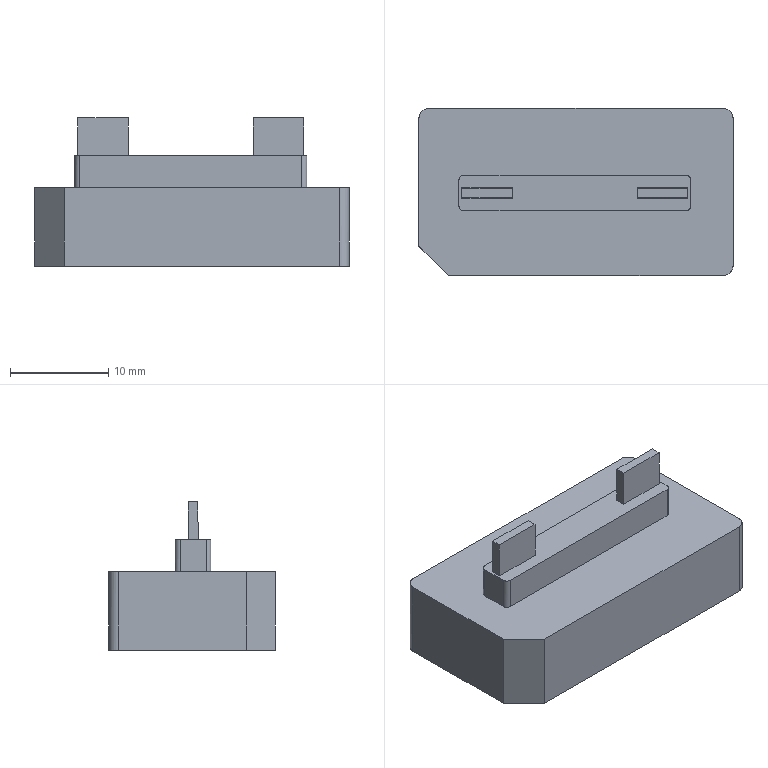NC program | PowerMill | posted by the shop | part box 32 x 17 x 15.109 mm
Lines 56306 to 56729 of 56729:
( TOOL ID   Text_D4_1_1 )
( TOOL DIA. 4. TIP RAD .3 LENGTH 62.36 )
( Z = -7.36 )
T13 M6
T1
G91 G28 Z0
G0 G90 G54
M08
S15000 M3
X0 Y0 M8
G43 Z10.299 H13
X-15.254 Y5.123
Z-7.26
G1 Z-7.36
X-15.245 Y5.357 F1000
X-15.219 Y5.563
X-15.175 Y5.741
X-15.114 Y5.893
X-15.035 Y6.016
X-14.938 Y6.112
X-14.825 Y6.181
X-14.693 Y6.222
X-14.544 Y6.236
X-14.395 Y6.222
X-14.264 Y6.181
X-14.15 Y6.112
X-14.053 Y6.016
X-13.974 Y5.893
X-13.913 Y5.741
X-13.869 Y5.563
X-13.843 Y5.357
X-13.834 Y5.123
X-13.843 Y4.894
X-13.869 Y4.692
X-13.913 Y4.515
X-13.974 Y4.365
X-14.053 Y4.24
X-14.149 Y4.141
X-14.262 Y4.07
X-14.394 Y4.028
X-14.544 Y4.014
X-14.693 Y4.027
X-14.825 Y4.068
X-14.938 Y4.137
X-15.035 Y4.233
X-15.114 Y4.356
X-15.175 Y4.507
X-15.219 Y4.685
X-15.245 Y4.89
X-15.254 Y5.123
G0 Z-4.242
G1 X-12.208 Y5.221 F10000
G0 Z-7.26
G1 Z-7.36 F600
X-12.38 Y5.242 F1000
X-12.521 Y5.275
X-12.629 Y5.32
X-12.714 Y5.384
X-12.774 Y5.464
X-12.811 Y5.56
X-12.823 Y5.674
X-12.811 Y5.792
X-12.776 Y5.899
X-12.717 Y5.996
X-12.634 Y6.082
X-12.504 Y6.167
X-12.359 Y6.219
X-12.198 Y6.236
X-12.031 Y6.219
X-11.884 Y6.169
X-11.757 Y6.085
X-11.673 Y5.999
X-11.613 Y5.901
X-11.578 Y5.79
X-11.566 Y5.667
X-11.579 Y5.555
X-11.618 Y5.459
X-11.684 Y5.379
X-11.775 Y5.315
X-11.893 Y5.268
X-12.037 Y5.236
X-12.208 Y5.221
X-12.033 Y5.195
X-11.89 Y5.167
X-11.779 Y5.137
X-11.7 Y5.105
X-11.602 Y5.032
X-11.532 Y4.936
X-11.49 Y4.816
X-11.476 Y4.672
X-11.489 Y4.529
X-11.529 Y4.401
X-11.595 Y4.287
X-11.687 Y4.188
X-11.794 Y4.111
X-11.915 Y4.057
X-12.048 Y4.024
X-12.194 Y4.014
X-12.341 Y4.025
X-12.475 Y4.058
X-12.595 Y4.113
X-12.702 Y4.191
X-12.793 Y4.291
X-12.859 Y4.406
X-12.898 Y4.536
X-12.911 Y4.68
X-12.898 Y4.823
X-12.859 Y4.941
X-12.793 Y5.035
X-12.702 Y5.105
X-12.629 Y5.135
X-12.523 Y5.165
X-12.382 Y5.193
X-12.208 Y5.221
G0 Z-4.242
G1 X-9.768 Y4.818 F10000
G0 Z-7.26
G1 Z-7.36 F600
X-10.603 F1000
G0 Z-4.242
G1 X-8.884 Y4.89 F10000
G0 Z-7.26
G1 Z-7.36 F600
X-8.893 Y5.123 F1000
X-8.884 Y5.357
X-8.858 Y5.563
X-8.814 Y5.741
X-8.753 Y5.893
X-8.674 Y6.016
X-8.578 Y6.112
X-8.464 Y6.181
X-8.332 Y6.222
X-8.183 Y6.236
X-8.034 Y6.222
X-7.903 Y6.181
X-7.789 Y6.112
X-7.692 Y6.016
X-7.614 Y5.893
X-7.552 Y5.741
X-7.508 Y5.563
X-7.482 Y5.357
X-7.473 Y5.123
X-7.482 Y4.894
X-7.508 Y4.692
X-7.552 Y4.515
X-7.613 Y4.365
X-7.692 Y4.24
X-7.789 Y4.141
X-7.902 Y4.07
X-8.033 Y4.028
X-8.183 Y4.014
X-8.332 Y4.027
X-8.464 Y4.068
X-8.578 Y4.137
X-8.674 Y4.233
X-8.753 Y4.356
X-8.814 Y4.507
X-8.858 Y4.685
X-8.884 Y4.89
G0 Z-4.242
G1 X-6.552 Y4.901 F10000
G0 Z-7.26
G1 Z-7.36 F600
X-6.457 Y5.047 F1000
X-6.349 Y5.175
X-6.227 Y5.286
X-6.075 Y5.383
X-5.921 Y5.442
X-5.766 Y5.461
X-5.628 Y5.448
X-5.504 Y5.408
X-5.393 Y5.342
X-5.296 Y5.249
X-5.221 Y5.143
X-5.167 Y5.026
X-5.134 Y4.897
X-5.124 Y4.757
X-5.135 Y4.606
X-5.169 Y4.469
X-5.226 Y4.345
X-5.306 Y4.234
X-5.409 Y4.138
X-5.526 Y4.069
X-5.658 Y4.027
X-5.804 Y4.014
X-5.962 Y4.027
X-6.102 Y4.066
X-6.224 Y4.131
X-6.327 Y4.222
X-6.411 Y4.339
X-6.476 Y4.482
X-6.523 Y4.652
X-6.551 Y4.847
X-6.56 Y5.068
X-6.55 Y5.313
X-6.521 Y5.53
X-6.473 Y5.717
X-6.406 Y5.876
X-6.319 Y6.005
X-6.213 Y6.106
X-6.087 Y6.178
X-5.943 Y6.222
X-5.779 Y6.236
X-5.618 Y6.22
X-5.478 Y6.172
X-5.358 Y6.092
X-5.264 Y5.983
X-5.198 Y5.851
X-5.162 Y5.694
G0 Z-4.242
G1 X-3.605 Y5.944 F10000
G0 Z-7.26
G1 Z-7.36 F600
X-3.195 Y6.226 F1000
Y4.05
G0 Z-4.242
G1 X-1.851 Y4.617 F10000
G0 Z-7.26
G1 Z-7.36 F600
X-1.815 Y4.457 F1000
X-1.758 Y4.322
X-1.68 Y4.211
X-1.581 Y4.124
X-1.461 Y4.063
X-1.32 Y4.026
X-1.157 Y4.014
X-.985 Y4.033
X-.822 Y4.091
X-.668 Y4.188
X-.566 Y4.284
X-.492 Y4.389
X-.447 Y4.502
X-.431 Y4.624
X-.441 Y4.799
X-.474 Y4.943
X-.529 Y5.055
X-.608 Y5.135
X-.688 Y5.176
X-.797 Y5.206
X-.934 Y5.223
X-1.099 Y5.229
X-1.401 Y5.228
X-.839
X-.731 Y5.289
X-.648 Y5.365
X-.588 Y5.455
X-.552 Y5.56
X-.54 Y5.68
X-.552 Y5.796
X-.587 Y5.902
X-.645 Y5.997
X-.726 Y6.082
X-.851 Y6.167
X-.991 Y6.217
X-1.147 Y6.234
X-1.312 Y6.221
X-1.455 Y6.18
X-1.577 Y6.113
X-1.677 Y6.019
X-1.756 Y5.898
X-1.792 Y5.803
X-1.824 Y5.675
G0 Z-4.242
G1 X1.285 Y4.818 F10000
G0 Z-7.26
G1 Z-7.36 F600
X.451 F1000
G0 Z-4.242
G1 X2.164 Y4.617 F10000
G0 Z-7.26
G1 Z-7.36 F600
X2.199 Y4.457 F1000
X2.256 Y4.322
X2.334 Y4.211
X2.433 Y4.124
X2.553 Y4.063
X2.695 Y4.026
X2.857 Y4.014
X3.029 Y4.033
X3.192 Y4.091
X3.346 Y4.188
X3.449 Y4.284
X3.523 Y4.389
X3.567 Y4.502
X3.584 Y4.624
X3.574 Y4.799
X3.541 Y4.943
X3.485 Y5.055
X3.406 Y5.135
X3.326 Y5.176
X3.218 Y5.206
X3.081 Y5.223
X2.915 Y5.229
X2.613 Y5.228
X3.176
X3.283 Y5.289
X3.367 Y5.365
X3.426 Y5.455
X3.462 Y5.56
X3.474 Y5.68
X3.462 Y5.796
X3.428 Y5.902
X3.37 Y5.997
X3.288 Y6.082
X3.163 Y6.167
X3.023 Y6.217
X2.867 Y6.234
X2.703 Y6.221
X2.559 Y6.18
X2.438 Y6.113
X2.337 Y6.019
X2.258 Y5.898
X2.222 Y5.803
X2.19 Y5.675
G0 Z-4.242
G1 X5.3 Y4.818 F10000
G0 Z-7.26
G1 Z-7.36 F600
X4.465 F1000
G0 Z-4.242
G1 X6.184 Y4.89 F10000
G0 Z-7.26
G1 Z-7.36 F600
X6.175 Y5.123 F1000
X6.184 Y5.357
X6.21 Y5.563
X6.254 Y5.741
X6.315 Y5.893
X6.394 Y6.016
X6.49 Y6.112
X6.604 Y6.181
X6.736 Y6.222
X6.885 Y6.236
X7.034 Y6.222
X7.165 Y6.181
X7.279 Y6.112
X7.376 Y6.016
X7.454 Y5.893
X7.516 Y5.741
X7.56 Y5.563
X7.586 Y5.357
X7.595 Y5.123
X7.586 Y4.894
X7.56 Y4.692
X7.516 Y4.515
X7.455 Y4.365
X7.376 Y4.24
X7.28 Y4.141
X7.166 Y4.07
X7.035 Y4.028
X6.885 Y4.014
X6.736 Y4.027
X6.604 Y4.068
X6.49 Y4.137
X6.394 Y4.233
X6.315 Y4.356
X6.254 Y4.507
X6.21 Y4.685
X6.184 Y4.89
G0 Z-4.242
G1 X8.805 Y4.159 F10000
G0 Z-7.26
G1 Z-7.36 F600
Y4.461 F1000
G0 Z-4.242
G1 X10.057 Y4.685 F10000
G0 Z-7.26
G1 Z-7.36 F600
X10.031 Y4.89 F1000
X10.022 Y5.123
X10.031 Y5.357
X10.057 Y5.563
X10.101 Y5.741
X10.162 Y5.893
X10.241 Y6.016
X10.337 Y6.112
X10.451 Y6.181
X10.583 Y6.222
X10.732 Y6.236
X10.881 Y6.222
X11.012 Y6.181
X11.126 Y6.112
X11.222 Y6.016
X11.301 Y5.893
X11.363 Y5.741
X11.407 Y5.563
X11.433 Y5.357
X11.442 Y5.123
X11.433 Y4.894
X11.407 Y4.692
X11.363 Y4.515
X11.302 Y4.365
X11.223 Y4.24
X11.126 Y4.141
X11.013 Y4.07
X10.882 Y4.028
X10.732 Y4.014
X10.583 Y4.027
X10.451 Y4.068
X10.337 Y4.137
X10.241 Y4.233
X10.162 Y4.356
X10.101 Y4.507
X10.057 Y4.685
G0 Z-4.242
G1 X12.385 Y6.198 F10000
G0 Z-7.26
G1 Z-7.36 F600
X13.793 F1000
X13.752 Y6.08
X13.69 Y5.945
X13.609 Y5.791
X13.382 Y5.402
X13.247 Y5.134
X13.137 Y4.865
X13.054 Y4.595
X12.996 Y4.323
X12.964 Y4.05
G0 Z10.299
M9
G91 G28 Z0
M5
M30
%